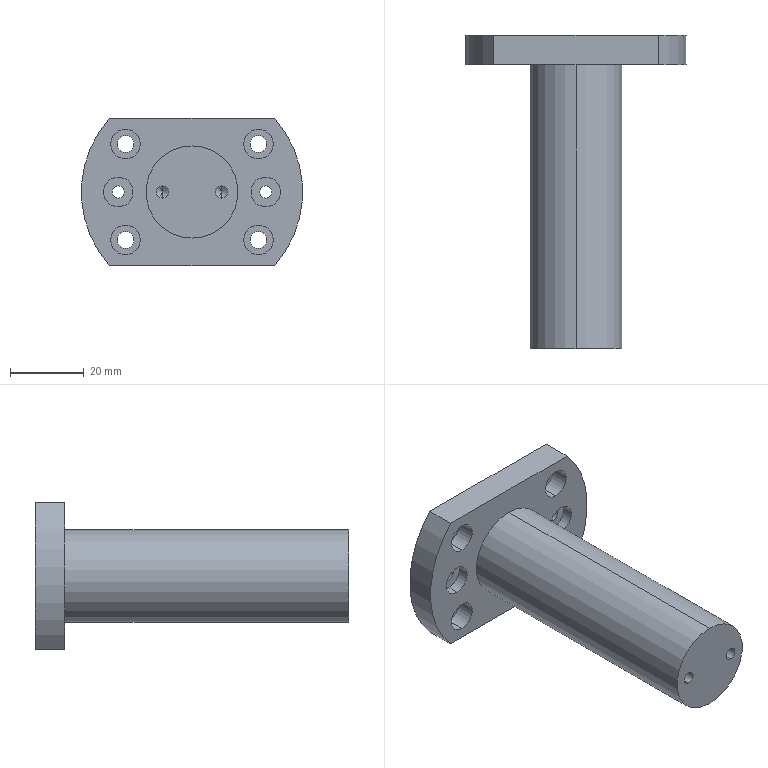Part | SolidWorks | features 3DProfileFeature 4, HoleWzd 4, ICE 1, Revolution 1 | 1 solid | 47 faces | box 60 x 85 x 40 mm | volume 53675 mm3 | cylinder 32 | plane 11 | cone 4 | commonest cylinder face diameters 8 x12 3.3 x8 4.5 x8 25 x2 60 x2
STEP:
#1=CARTESIAN_POINT('',(-18.,82.,17.));
#2=VERTEX_POINT('',#1);
#3=CARTESIAN_POINT('',(-18.,82.,9.));
#4=VERTEX_POINT('',#3);
#5=CARTESIAN_POINT('',(-18.,82.,13.));
#6=DIRECTION('',(0.,-1.,0.));
#7=DIRECTION('',(0.,0.,-1.));
#8=AXIS2_PLACEMENT_3D('',#5,#6,#7);
#9=CIRCLE('',#8,4.);
#10=EDGE_CURVE('',#2,#4,#9,.T.);
#11=ORIENTED_EDGE('',*,*,#10,.F.);
#12=CARTESIAN_POINT('',(-18.,77.,17.));
#13=VERTEX_POINT('',#12);
#14=CARTESIAN_POINT('',(-18.,77.,17.));
#15=DIRECTION('',(0.,-1.,0.));
#16=VECTOR('',#15,1000.);
#17=LINE('',#14,#16);
#18=EDGE_CURVE('',#2,#13,#17,.T.);
#19=ORIENTED_EDGE('',*,*,#18,.T.);
#20=CARTESIAN_POINT('',(-18.,77.,9.));
#21=VERTEX_POINT('',#20);
#22=CARTESIAN_POINT('',(-18.,77.,13.));
#23=DIRECTION('',(0.,-1.,0.));
#24=DIRECTION('',(0.,0.,-1.));
#25=AXIS2_PLACEMENT_3D('',#22,#23,#24);
#26=CIRCLE('',#25,4.);
#27=EDGE_CURVE('',#13,#21,#26,.T.);
#28=ORIENTED_EDGE('',*,*,#27,.T.);
#29=CARTESIAN_POINT('',(-18.,77.,9.));
#30=DIRECTION('',(0.,-1.,0.));
#31=VECTOR('',#30,1000.);
#32=LINE('',#29,#31);
#33=EDGE_CURVE('',#4,#21,#32,.T.);
#34=ORIENTED_EDGE('',*,*,#33,.F.);
#35=EDGE_LOOP('',(#11,#19,#28,#34));
#36=FACE_OUTER_BOUND('',#35,.T.);
#37=CARTESIAN_POINT('',(-18.,77.,13.));
#38=DIRECTION('',(0.,-1.,0.));
#39=DIRECTION('',(0.,0.,-1.));
#40=AXIS2_PLACEMENT_3D('',#37,#38,#39);
#41=CYLINDRICAL_SURFACE('',#40,4.);
#42=ADVANCED_FACE('',(#36),#41,.F.);
#43=CARTESIAN_POINT('',(-18.,85.,15.25));
#44=VERTEX_POINT('',#43);
#45=CARTESIAN_POINT('',(-18.,85.,10.75));
#46=VERTEX_POINT('',#45);
#47=CARTESIAN_POINT('',(-18.,85.,13.));
#48=DIRECTION('',(0.,-1.,0.));
#49=DIRECTION('',(0.,0.,-1.));
#50=AXIS2_PLACEMENT_3D('',#47,#48,#49);
#51=CIRCLE('',#50,2.25);
#52=EDGE_CURVE('',#44,#46,#51,.T.);
#53=ORIENTED_EDGE('',*,*,#52,.F.);
#54=CARTESIAN_POINT('',(-18.,82.,15.25));
#55=VERTEX_POINT('',#54);
#56=CARTESIAN_POINT('',(-18.,77.,15.25));
#57=DIRECTION('',(0.,-1.,0.));
#58=VECTOR('',#57,1000.);
#59=LINE('',#56,#58);
#60=EDGE_CURVE('',#44,#55,#59,.T.);
#61=ORIENTED_EDGE('',*,*,#60,.T.);
#62=CARTESIAN_POINT('',(-18.,82.,10.75));
#63=VERTEX_POINT('',#62);
#64=CARTESIAN_POINT('',(-18.,82.,13.));
#65=DIRECTION('',(0.,-1.,0.));
#66=DIRECTION('',(0.,0.,-1.));
#67=AXIS2_PLACEMENT_3D('',#64,#65,#66);
#68=CIRCLE('',#67,2.25);
#69=EDGE_CURVE('',#55,#63,#68,.T.);
#70=ORIENTED_EDGE('',*,*,#69,.T.);
#71=CARTESIAN_POINT('',(-18.,77.,10.75));
#72=DIRECTION('',(0.,-1.,0.));
#73=VECTOR('',#72,1000.);
#74=LINE('',#71,#73);
#75=EDGE_CURVE('',#46,#63,#74,.T.);
#76=ORIENTED_EDGE('',*,*,#75,.F.);
#77=EDGE_LOOP('',(#53,#61,#70,#76));
#78=FACE_OUTER_BOUND('',#77,.T.);
#79=CARTESIAN_POINT('',(-18.,77.,13.));
#80=DIRECTION('',(0.,-1.,0.));
#81=DIRECTION('',(0.,0.,-1.));
#82=AXIS2_PLACEMENT_3D('',#79,#80,#81);
#83=CYLINDRICAL_SURFACE('',#82,2.25);
#84=ADVANCED_FACE('',(#78),#83,.F.);
#85=CARTESIAN_POINT('',(18.,82.,17.));
#86=VERTEX_POINT('',#85);
#87=CARTESIAN_POINT('',(18.,82.,9.));
#88=VERTEX_POINT('',#87);
#89=CARTESIAN_POINT('',(18.,82.,13.));
#90=DIRECTION('',(0.,-1.,0.));
#91=DIRECTION('',(0.,0.,-1.));
#92=AXIS2_PLACEMENT_3D('',#89,#90,#91);
#93=CIRCLE('',#92,4.);
#94=EDGE_CURVE('',#86,#88,#93,.T.);
#95=ORIENTED_EDGE('',*,*,#94,.F.);
#96=CARTESIAN_POINT('',(18.,77.,17.));
#97=VERTEX_POINT('',#96);
#98=CARTESIAN_POINT('',(18.,77.,17.));
#99=DIRECTION('',(0.,-1.,0.));
#100=VECTOR('',#99,1000.);
#101=LINE('',#98,#100);
#102=EDGE_CURVE('',#86,#97,#101,.T.);
#103=ORIENTED_EDGE('',*,*,#102,.T.);
#104=CARTESIAN_POINT('',(18.,77.,9.));
#105=VERTEX_POINT('',#104);
#106=CARTESIAN_POINT('',(18.,77.,13.));
#107=DIRECTION('',(0.,-1.,0.));
#108=DIRECTION('',(0.,0.,-1.));
#109=AXIS2_PLACEMENT_3D('',#106,#107,#108);
#110=CIRCLE('',#109,4.);
#111=EDGE_CURVE('',#97,#105,#110,.T.);
#112=ORIENTED_EDGE('',*,*,#111,.T.);
#113=CARTESIAN_POINT('',(18.,77.,9.));
#114=DIRECTION('',(0.,-1.,0.));
#115=VECTOR('',#114,1000.);
#116=LINE('',#113,#115);
#117=EDGE_CURVE('',#88,#105,#116,.T.);
#118=ORIENTED_EDGE('',*,*,#117,.F.);
#119=EDGE_LOOP('',(#95,#103,#112,#118));
#120=FACE_OUTER_BOUND('',#119,.T.);
#121=CARTESIAN_POINT('',(18.,77.,13.));
#122=DIRECTION('',(0.,-1.,0.));
#123=DIRECTION('',(0.,0.,-1.));
#124=AXIS2_PLACEMENT_3D('',#121,#122,#123);
#125=CYLINDRICAL_SURFACE('',#124,4.);
#126=ADVANCED_FACE('',(#120),#125,.F.);
#127=CARTESIAN_POINT('',(18.,85.,15.25));
#128=VERTEX_POINT('',#127);
#129=CARTESIAN_POINT('',(18.,85.,10.75));
#130=VERTEX_POINT('',#129);
#131=CARTESIAN_POINT('',(18.,85.,13.));
#132=DIRECTION('',(0.,-1.,0.));
#133=DIRECTION('',(0.,0.,-1.));
#134=AXIS2_PLACEMENT_3D('',#131,#132,#133);
#135=CIRCLE('',#134,2.25);
#136=EDGE_CURVE('',#128,#130,#135,.T.);
#137=ORIENTED_EDGE('',*,*,#136,.F.);
#138=CARTESIAN_POINT('',(18.,82.,15.25));
#139=VERTEX_POINT('',#138);
#140=CARTESIAN_POINT('',(18.,77.,15.25));
#141=DIRECTION('',(0.,-1.,0.));
#142=VECTOR('',#141,1000.);
#143=LINE('',#140,#142);
#144=EDGE_CURVE('',#128,#139,#143,.T.);
#145=ORIENTED_EDGE('',*,*,#144,.T.);
#146=CARTESIAN_POINT('',(18.,82.,10.75));
#147=VERTEX_POINT('',#146);
#148=CARTESIAN_POINT('',(18.,82.,13.));
#149=DIRECTION('',(0.,-1.,0.));
#150=DIRECTION('',(0.,0.,-1.));
#151=AXIS2_PLACEMENT_3D('',#148,#149,#150);
#152=CIRCLE('',#151,2.25);
#153=EDGE_CURVE('',#139,#147,#152,.T.);
#154=ORIENTED_EDGE('',*,*,#153,.T.);
#155=CARTESIAN_POINT('',(18.,77.,10.75));
#156=DIRECTION('',(0.,-1.,0.));
#157=VECTOR('',#156,1000.);
#158=LINE('',#155,#157);
#159=EDGE_CURVE('',#130,#147,#158,.T.);
#160=ORIENTED_EDGE('',*,*,#159,.F.);
#161=EDGE_LOOP('',(#137,#145,#154,#160));
#162=FACE_OUTER_BOUND('',#161,.T.);
#163=CARTESIAN_POINT('',(18.,77.,13.));
#164=DIRECTION('',(0.,-1.,0.));
#165=DIRECTION('',(0.,0.,-1.));
#166=AXIS2_PLACEMENT_3D('',#163,#164,#165);
#167=CYLINDRICAL_SURFACE('',#166,2.25);
#168=ADVANCED_FACE('',(#162),#167,.F.);
#169=CARTESIAN_POINT('',(18.,82.,-9.));
#170=VERTEX_POINT('',#169);
#171=CARTESIAN_POINT('',(18.,82.,-17.));
#172=VERTEX_POINT('',#171);
#173=CARTESIAN_POINT('',(18.,82.,-13.));
#174=DIRECTION('',(0.,-1.,0.));
#175=DIRECTION('',(0.,0.,-1.));
#176=AXIS2_PLACEMENT_3D('',#173,#174,#175);
#177=CIRCLE('',#176,4.);
#178=EDGE_CURVE('',#170,#172,#177,.T.);
#179=ORIENTED_EDGE('',*,*,#178,.F.);
#180=CARTESIAN_POINT('',(18.,77.,-9.));
#181=VERTEX_POINT('',#180);
#182=CARTESIAN_POINT('',(18.,77.,-9.));
#183=DIRECTION('',(0.,-1.,0.));
#184=VECTOR('',#183,1000.);
#185=LINE('',#182,#184);
#186=EDGE_CURVE('',#170,#181,#185,.T.);
#187=ORIENTED_EDGE('',*,*,#186,.T.);
#188=CARTESIAN_POINT('',(18.,77.,-17.));
#189=VERTEX_POINT('',#188);
#190=CARTESIAN_POINT('',(18.,77.,-13.));
#191=DIRECTION('',(0.,-1.,0.));
#192=DIRECTION('',(0.,0.,-1.));
#193=AXIS2_PLACEMENT_3D('',#190,#191,#192);
#194=CIRCLE('',#193,4.);
#195=EDGE_CURVE('',#181,#189,#194,.T.);
#196=ORIENTED_EDGE('',*,*,#195,.T.);
#197=CARTESIAN_POINT('',(18.,77.,-17.));
#198=DIRECTION('',(0.,-1.,0.));
#199=VECTOR('',#198,1000.);
#200=LINE('',#197,#199);
#201=EDGE_CURVE('',#172,#189,#200,.T.);
#202=ORIENTED_EDGE('',*,*,#201,.F.);
#203=EDGE_LOOP('',(#179,#187,#196,#202));
#204=FACE_OUTER_BOUND('',#203,.T.);
#205=CARTESIAN_POINT('',(18.,77.,-13.));
#206=DIRECTION('',(0.,-1.,0.));
#207=DIRECTION('',(0.,0.,-1.));
#208=AXIS2_PLACEMENT_3D('',#205,#206,#207);
#209=CYLINDRICAL_SURFACE('',#208,4.);
#210=ADVANCED_FACE('',(#204),#209,.F.);
#211=CARTESIAN_POINT('',(18.,85.,-10.75));
#212=VERTEX_POINT('',#211);
#213=CARTESIAN_POINT('',(18.,85.,-15.25));
#214=VERTEX_POINT('',#213);
#215=CARTESIAN_POINT('',(18.,85.,-13.));
#216=DIRECTION('',(0.,-1.,0.));
#217=DIRECTION('',(0.,0.,-1.));
#218=AXIS2_PLACEMENT_3D('',#215,#216,#217);
#219=CIRCLE('',#218,2.25);
#220=EDGE_CURVE('',#212,#214,#219,.T.);
#221=ORIENTED_EDGE('',*,*,#220,.F.);
#222=CARTESIAN_POINT('',(18.,82.,-10.75));
#223=VERTEX_POINT('',#222);
#224=CARTESIAN_POINT('',(18.,77.,-10.75));
#225=DIRECTION('',(0.,-1.,0.));
#226=VECTOR('',#225,1000.);
#227=LINE('',#224,#226);
#228=EDGE_CURVE('',#212,#223,#227,.T.);
#229=ORIENTED_EDGE('',*,*,#228,.T.);
#230=CARTESIAN_POINT('',(18.,82.,-15.25));
#231=VERTEX_POINT('',#230);
#232=CARTESIAN_POINT('',(18.,82.,-13.));
#233=DIRECTION('',(0.,-1.,0.));
#234=DIRECTION('',(0.,0.,-1.));
#235=AXIS2_PLACEMENT_3D('',#232,#233,#234);
#236=CIRCLE('',#235,2.25);
#237=EDGE_CURVE('',#223,#231,#236,.T.);
#238=ORIENTED_EDGE('',*,*,#237,.T.);
#239=CARTESIAN_POINT('',(18.,77.,-15.25));
#240=DIRECTION('',(0.,-1.,0.));
#241=VECTOR('',#240,1000.);
#242=LINE('',#239,#241);
#243=EDGE_CURVE('',#214,#231,#242,.T.);
#244=ORIENTED_EDGE('',*,*,#243,.F.);
#245=EDGE_LOOP('',(#221,#229,#238,#244));
#246=FACE_OUTER_BOUND('',#245,.T.);
#247=CARTESIAN_POINT('',(18.,77.,-13.));
#248=DIRECTION('',(0.,-1.,0.));
#249=DIRECTION('',(0.,0.,-1.));
#250=AXIS2_PLACEMENT_3D('',#247,#248,#249);
#251=CYLINDRICAL_SURFACE('',#250,2.25);
#252=ADVANCED_FACE('',(#246),#251,.F.);
#253=CARTESIAN_POINT('',(-18.,82.,-9.));
#254=VERTEX_POINT('',#253);
#255=CARTESIAN_POINT('',(-18.,82.,-17.));
#256=VERTEX_POINT('',#255);
#257=CARTESIAN_POINT('',(-18.,82.,-13.));
#258=DIRECTION('',(0.,-1.,0.));
#259=DIRECTION('',(0.,0.,-1.));
#260=AXIS2_PLACEMENT_3D('',#257,#258,#259);
#261=CIRCLE('',#260,4.);
#262=EDGE_CURVE('',#254,#256,#261,.T.);
#263=ORIENTED_EDGE('',*,*,#262,.F.);
#264=CARTESIAN_POINT('',(-18.,77.,-9.));
#265=VERTEX_POINT('',#264);
#266=CARTESIAN_POINT('',(-18.,77.,-9.));
#267=DIRECTION('',(0.,-1.,0.));
#268=VECTOR('',#267,1000.);
#269=LINE('',#266,#268);
#270=EDGE_CURVE('',#254,#265,#269,.T.);
#271=ORIENTED_EDGE('',*,*,#270,.T.);
#272=CARTESIAN_POINT('',(-18.,77.,-17.));
#273=VERTEX_POINT('',#272);
#274=CARTESIAN_POINT('',(-18.,77.,-13.));
#275=DIRECTION('',(0.,-1.,0.));
#276=DIRECTION('',(0.,0.,-1.));
#277=AXIS2_PLACEMENT_3D('',#274,#275,#276);
#278=CIRCLE('',#277,4.);
#279=EDGE_CURVE('',#265,#273,#278,.T.);
#280=ORIENTED_EDGE('',*,*,#279,.T.);
#281=CARTESIAN_POINT('',(-18.,77.,-17.));
#282=DIRECTION('',(0.,-1.,0.));
#283=VECTOR('',#282,1000.);
#284=LINE('',#281,#283);
#285=EDGE_CURVE('',#256,#273,#284,.T.);
#286=ORIENTED_EDGE('',*,*,#285,.F.);
#287=EDGE_LOOP('',(#263,#271,#280,#286));
#288=FACE_OUTER_BOUND('',#287,.T.);
#289=CARTESIAN_POINT('',(-18.,77.,-13.));
#290=DIRECTION('',(0.,-1.,0.));
#291=DIRECTION('',(0.,0.,-1.));
#292=AXIS2_PLACEMENT_3D('',#289,#290,#291);
#293=CYLINDRICAL_SURFACE('',#292,4.);
#294=ADVANCED_FACE('',(#288),#293,.F.);
#295=CARTESIAN_POINT('',(-18.,85.,-10.75));
#296=VERTEX_POINT('',#295);
#297=CARTESIAN_POINT('',(-18.,85.,-15.25));
#298=VERTEX_POINT('',#297);
#299=CARTESIAN_POINT('',(-18.,85.,-13.));
#300=DIRECTION('',(0.,-1.,0.));
#301=DIRECTION('',(0.,0.,-1.));
#302=AXIS2_PLACEMENT_3D('',#299,#300,#301);
#303=CIRCLE('',#302,2.25);
#304=EDGE_CURVE('',#296,#298,#303,.T.);
#305=ORIENTED_EDGE('',*,*,#304,.F.);
#306=CARTESIAN_POINT('',(-18.,82.,-10.75));
#307=VERTEX_POINT('',#306);
#308=CARTESIAN_POINT('',(-18.,77.,-10.75));
#309=DIRECTION('',(0.,-1.,0.));
#310=VECTOR('',#309,1000.);
#311=LINE('',#308,#310);
#312=EDGE_CURVE('',#296,#307,#311,.T.);
#313=ORIENTED_EDGE('',*,*,#312,.T.);
#314=CARTESIAN_POINT('',(-18.,82.,-15.25));
#315=VERTEX_POINT('',#314);
#316=CARTESIAN_POINT('',(-18.,82.,-13.));
#317=DIRECTION('',(0.,-1.,0.));
#318=DIRECTION('',(0.,0.,-1.));
#319=AXIS2_PLACEMENT_3D('',#316,#317,#318);
#320=CIRCLE('',#319,2.25);
#321=EDGE_CURVE('',#307,#315,#320,.T.);
#322=ORIENTED_EDGE('',*,*,#321,.T.);
#323=CARTESIAN_POINT('',(-18.,77.,-15.25));
#324=DIRECTION('',(0.,-1.,0.));
#325=VECTOR('',#324,1000.);
#326=LINE('',#323,#325);
#327=EDGE_CURVE('',#298,#315,#326,.T.);
#328=ORIENTED_EDGE('',*,*,#327,.F.);
#329=EDGE_LOOP('',(#305,#313,#322,#328));
#330=FACE_OUTER_BOUND('',#329,.T.);
#331=CARTESIAN_POINT('',(-18.,77.,-13.));
#332=DIRECTION('',(0.,-1.,0.));
#333=DIRECTION('',(0.,0.,-1.));
#334=AXIS2_PLACEMENT_3D('',#331,#332,#333);
#335=CYLINDRICAL_SURFACE('',#334,2.25);
#336=ADVANCED_FACE('',(#330),#335,.F.);
#337=CARTESIAN_POINT('',(-20.,85.,1.65));
#338=VERTEX_POINT('',#337);
#339=CARTESIAN_POINT('',(-20.,85.,-1.65));
#340=VERTEX_POINT('',#339);
#341=CARTESIAN_POINT('',(-20.,85.,0.));
#342=DIRECTION('',(0.,-1.,0.));
#343=DIRECTION('',(0.,0.,-1.));
#344=AXIS2_PLACEMENT_3D('',#341,#342,#343);
#345=CIRCLE('',#344,1.65);
#346=EDGE_CURVE('',#338,#340,#345,.T.);
#347=ORIENTED_EDGE('',*,*,#346,.F.);
#348=CARTESIAN_POINT('',(-20.,80.,1.65));
#349=VERTEX_POINT('',#348);
#350=CARTESIAN_POINT('',(-20.,80.,1.65));
#351=DIRECTION('',(0.,-1.,0.));
#352=VECTOR('',#351,1000.);
#353=LINE('',#350,#352);
#354=EDGE_CURVE('',#338,#349,#353,.T.);
#355=ORIENTED_EDGE('',*,*,#354,.T.);
#356=CARTESIAN_POINT('',(-20.,80.,-1.65));
#357=VERTEX_POINT('',#356);
#358=CARTESIAN_POINT('',(-20.,80.,0.));
#359=DIRECTION('',(0.,-1.,0.));
#360=DIRECTION('',(0.,0.,-1.));
#361=AXIS2_PLACEMENT_3D('',#358,#359,#360);
#362=CIRCLE('',#361,1.65);
#363=EDGE_CURVE('',#349,#357,#362,.T.);
#364=ORIENTED_EDGE('',*,*,#363,.T.);
#365=CARTESIAN_POINT('',(-20.,80.,-1.65));
#366=DIRECTION('',(0.,-1.,0.));
#367=VECTOR('',#366,1000.);
#368=LINE('',#365,#367);
#369=EDGE_CURVE('',#340,#357,#368,.T.);
#370=ORIENTED_EDGE('',*,*,#369,.F.);
#371=EDGE_LOOP('',(#347,#355,#364,#370));
#372=FACE_OUTER_BOUND('',#371,.T.);
#373=CARTESIAN_POINT('',(-20.,80.,0.));
#374=DIRECTION('',(0.,-1.,0.));
#375=DIRECTION('',(0.,0.,-1.));
#376=AXIS2_PLACEMENT_3D('',#373,#374,#375);
#377=CYLINDRICAL_SURFACE('',#376,1.65);
#378=ADVANCED_FACE('',(#372),#377,.F.);
#379=CARTESIAN_POINT('',(20.,85.,1.65));
#380=VERTEX_POINT('',#379);
#381=CARTESIAN_POINT('',(20.,85.,-1.65));
#382=VERTEX_POINT('',#381);
#383=CARTESIAN_POINT('',(20.,85.,0.));
#384=DIRECTION('',(0.,-1.,0.));
#385=DIRECTION('',(0.,0.,-1.));
#386=AXIS2_PLACEMENT_3D('',#383,#384,#385);
#387=CIRCLE('',#386,1.65);
#388=EDGE_CURVE('',#380,#382,#387,.T.);
#389=ORIENTED_EDGE('',*,*,#388,.F.);
#390=CARTESIAN_POINT('',(20.,80.,1.65));
#391=VERTEX_POINT('',#390);
#392=CARTESIAN_POINT('',(20.,80.,1.65));
#393=DIRECTION('',(0.,-1.,0.));
#394=VECTOR('',#393,1000.);
#395=LINE('',#392,#394);
#396=EDGE_CURVE('',#380,#391,#395,.T.);
#397=ORIENTED_EDGE('',*,*,#396,.T.);
#398=CARTESIAN_POINT('',(20.,80.,-1.65));
#399=VERTEX_POINT('',#398);
#400=CARTESIAN_POINT('',(20.,80.,0.));
#401=DIRECTION('',(0.,-1.,0.));
#402=DIRECTION('',(0.,0.,-1.));
#403=AXIS2_PLACEMENT_3D('',#400,#401,#402);
#404=CIRCLE('',#403,1.65);
#405=EDGE_CURVE('',#391,#399,#404,.T.);
#406=ORIENTED_EDGE('',*,*,#405,.T.);
#407=CARTESIAN_POINT('',(20.,80.,-1.65));
#408=DIRECTION('',(0.,-1.,0.));
#409=VECTOR('',#408,1000.);
#410=LINE('',#407,#409);
#411=EDGE_CURVE('',#382,#399,#410,.T.);
#412=ORIENTED_EDGE('',*,*,#411,.F.);
#413=EDGE_LOOP('',(#389,#397,#406,#412));
#414=FACE_OUTER_BOUND('',#413,.T.);
#415=CARTESIAN_POINT('',(20.,80.,0.));
#416=DIRECTION('',(0.,-1.,0.));
#417=DIRECTION('',(0.,0.,-1.));
#418=AXIS2_PLACEMENT_3D('',#415,#416,#417);
#419=CYLINDRICAL_SURFACE('',#418,1.65);
#420=ADVANCED_FACE('',(#414),#419,.F.);
#421=CARTESIAN_POINT('',(-20.,80.,4.));
#422=VERTEX_POINT('',#421);
#423=CARTESIAN_POINT('',(-20.,80.,-4.));
#424=VERTEX_POINT('',#423);
#425=CARTESIAN_POINT('',(-20.,80.,0.));
#426=DIRECTION('',(0.,-1.,0.));
#427=DIRECTION('',(0.,0.,-1.));
#428=AXIS2_PLACEMENT_3D('',#425,#426,#427);
#429=CIRCLE('',#428,4.);
#430=EDGE_CURVE('',#422,#424,#429,.T.);
#431=ORIENTED_EDGE('',*,*,#430,.F.);
#432=CARTESIAN_POINT('',(-20.,77.,4.));
#433=VERTEX_POINT('',#432);
#434=CARTESIAN_POINT('',(-20.,77.,4.));
#435=DIRECTION('',(0.,-1.,0.));
#436=VECTOR('',#435,1000.);
#437=LINE('',#434,#436);
#438=EDGE_CURVE('',#422,#433,#437,.T.);
#439=ORIENTED_EDGE('',*,*,#438,.T.);
#440=CARTESIAN_POINT('',(-20.,77.,-4.));
#441=VERTEX_POINT('',#440);
#442=CARTESIAN_POINT('',(-20.,77.,0.));
#443=DIRECTION('',(0.,-1.,0.));
#444=DIRECTION('',(0.,0.,-1.));
#445=AXIS2_PLACEMENT_3D('',#442,#443,#444);
#446=CIRCLE('',#445,4.);
#447=EDGE_CURVE('',#433,#441,#446,.T.);
#448=ORIENTED_EDGE('',*,*,#447,.T.);
#449=CARTESIAN_POINT('',(-20.,77.,-4.));
#450=DIRECTION('',(0.,-1.,0.));
#451=VECTOR('',#450,1000.);
#452=LINE('',#449,#451);
#453=EDGE_CURVE('',#424,#441,#452,.T.);
#454=ORIENTED_EDGE('',*,*,#453,.F.);
#455=EDGE_LOOP('',(#431,#439,#448,#454));
#456=FACE_OUTER_BOUND('',#455,.T.);
#457=CARTESIAN_POINT('',(-20.,77.,0.));
#458=DIRECTION('',(0.,-1.,0.));
#459=DIRECTION('',(0.,0.,-1.));
#460=AXIS2_PLACEMENT_3D('',#457,#458,#459);
#461=CYLINDRICAL_SURFACE('',#460,4.);
#462=ADVANCED_FACE('',(#456),#461,.F.);
#463=CARTESIAN_POINT('',(20.,80.,4.));
#464=VERTEX_POINT('',#463);
#465=CARTESIAN_POINT('',(20.,80.,-4.));
#466=VERTEX_POINT('',#465);
#467=CARTESIAN_POINT('',(20.,80.,0.));
#468=DIRECTION('',(0.,-1.,0.));
#469=DIRECTION('',(0.,0.,-1.));
#470=AXIS2_PLACEMENT_3D('',#467,#468,#469);
#471=CIRCLE('',#470,4.);
#472=EDGE_CURVE('',#464,#466,#471,.T.);
#473=ORIENTED_EDGE('',*,*,#472,.F.);
#474=CARTESIAN_POINT('',(20.,77.,4.));
#475=VERTEX_POINT('',#474);
#476=CARTESIAN_POINT('',(20.,77.,4.));
#477=DIRECTION('',(0.,-1.,0.));
#478=VECTOR('',#477,1000.);
#479=LINE('',#476,#478);
#480=EDGE_CURVE('',#464,#475,#479,.T.);
#481=ORIENTED_EDGE('',*,*,#480,.T.);
#482=CARTESIAN_POINT('',(20.,77.,-4.));
#483=VERTEX_POINT('',#482);
#484=CARTESIAN_POINT('',(20.,77.,0.));
#485=DIRECTION('',(0.,-1.,0.));
#486=DIRECTION('',(0.,0.,-1.));
#487=AXIS2_PLACEMENT_3D('',#484,#485,#486);
#488=CIRCLE('',#487,4.);
#489=EDGE_CURVE('',#475,#483,#488,.T.);
#490=ORIENTED_EDGE('',*,*,#489,.T.);
#491=CARTESIAN_POINT('',(20.,77.,-4.));
#492=DIRECTION('',(0.,-1.,0.));
#493=VECTOR('',#492,1000.);
#494=LINE('',#491,#493);
#495=EDGE_CURVE('',#466,#483,#494,.T.);
#496=ORIENTED_EDGE('',*,*,#495,.F.);
#497=EDGE_LOOP('',(#473,#481,#490,#496));
#498=FACE_OUTER_BOUND('',#497,.T.);
#499=CARTESIAN_POINT('',(20.,77.,0.));
#500=DIRECTION('',(0.,-1.,0.));
#501=DIRECTION('',(0.,0.,-1.));
#502=AXIS2_PLACEMENT_3D('',#499,#500,#501);
#503=CYLINDRICAL_SURFACE('',#502,4.);
#504=ADVANCED_FACE('',(#498),#503,.F.);
#505=CARTESIAN_POINT('',(-8.,11.5,1.65));
#506=VERTEX_POINT('',#505);
#507=CARTESIAN_POINT('',(-8.,11.5,-1.65));
#508=VERTEX_POINT('',#507);
#509=CARTESIAN_POINT('',(-8.,11.5,0.));
#510=DIRECTION('',(0.,-1.,0.));
#511=DIRECTION('',(0.,0.,-1.));
#512=AXIS2_PLACEMENT_3D('',#509,#510,#511);
#513=CIRCLE('',#512,1.65);
#514=EDGE_CURVE('',#506,#508,#513,.T.);
#515=ORIENTED_EDGE('',*,*,#514,.F.);
#516=CARTESIAN_POINT('',(-8.,0.,1.65));
#517=VERTEX_POINT('',#516);
#518=CARTESIAN_POINT('',(-8.,0.,1.65));
#519=DIRECTION('',(0.,-1.,0.));
#520=VECTOR('',#519,1000.);
#521=LINE('',#518,#520);
#522=EDGE_CURVE('',#506,#517,#521,.T.);
#523=ORIENTED_EDGE('',*,*,#522,.T.);
#524=CARTESIAN_POINT('',(-8.,0.,-1.65));
#525=VERTEX_POINT('',#524);
#526=CARTESIAN_POINT('',(-8.,0.,0.));
#527=DIRECTION('',(0.,-1.,0.));
#528=DIRECTION('',(0.,0.,-1.));
#529=AXIS2_PLACEMENT_3D('',#526,#527,#528);
#530=CIRCLE('',#529,1.65);
#531=EDGE_CURVE('',#517,#525,#530,.T.);
#532=ORIENTED_EDGE('',*,*,#531,.T.);
#533=CARTESIAN_POINT('',(-8.,0.,-1.65));
#534=DIRECTION('',(0.,-1.,0.));
#535=VECTOR('',#534,1000.);
#536=LINE('',#533,#535);
#537=EDGE_CURVE('',#508,#525,#536,.T.);
#538=ORIENTED_EDGE('',*,*,#537,.F.);
#539=EDGE_LOOP('',(#515,#523,#532,#538));
#540=FACE_OUTER_BOUND('',#539,.T.);
#541=CARTESIAN_POINT('',(-8.,0.,0.));
#542=DIRECTION('',(0.,-1.,0.));
#543=DIRECTION('',(0.,0.,-1.));
#544=AXIS2_PLACEMENT_3D('',#541,#542,#543);
#545=CYLINDRICAL_SURFACE('',#544,1.65);
#546=ADVANCED_FACE('',(#540),#545,.F.);
#547=CARTESIAN_POINT('',(-8.,12.491,0.));
#548=VERTEX_POINT('',#547);
#549=CARTESIAN_POINT('',(-8.,11.5,-1.65));
#550=DIRECTION('',(0.,-0.515,-0.8572));
#551=VECTOR('',#550,1000.);
#552=LINE('',#549,#551);
#553=EDGE_CURVE('',#548,#508,#552,.T.);
#554=ORIENTED_EDGE('',*,*,#553,.F.);
#555=CARTESIAN_POINT('',(-8.,11.5,1.65));
#556=DIRECTION('',(0.,-0.515,0.8572));
#557=VECTOR('',#556,1000.);
#558=LINE('',#555,#557);
#559=EDGE_CURVE('',#548,#506,#558,.T.);
#560=ORIENTED_EDGE('',*,*,#559,.T.);
#561=ORIENTED_EDGE('',*,*,#514,.T.);
#562=EDGE_LOOP('',(#554,#560,#561));
#563=FACE_OUTER_BOUND('',#562,.T.);
#564=CARTESIAN_POINT('',(-8.,11.5,0.));
#565=DIRECTION('',(0.,-1.,0.));
#566=DIRECTION('',(0.,0.,-1.));
#567=AXIS2_PLACEMENT_3D('',#564,#565,#566);
#568=CONICAL_SURFACE('',#567,1.65,1.03);
#569=ADVANCED_FACE('',(#563),#568,.F.);
#570=CARTESIAN_POINT('',(8.,11.5,1.65));
#571=VERTEX_POINT('',#570);
#572=CARTESIAN_POINT('',(8.,11.5,-1.65));
#573=VERTEX_POINT('',#572);
#574=CARTESIAN_POINT('',(8.,11.5,0.));
#575=DIRECTION('',(0.,-1.,0.));
#576=DIRECTION('',(0.,0.,-1.));
#577=AXIS2_PLACEMENT_3D('',#574,#575,#576);
#578=CIRCLE('',#577,1.65);
#579=EDGE_CURVE('',#571,#573,#578,.T.);
#580=ORIENTED_EDGE('',*,*,#579,.F.);
#581=CARTESIAN_POINT('',(8.,0.,1.65));
#582=VERTEX_POINT('',#581);
#583=CARTESIAN_POINT('',(8.,0.,1.65));
#584=DIRECTION('',(0.,-1.,0.));
#585=VECTOR('',#584,1000.);
#586=LINE('',#583,#585);
#587=EDGE_CURVE('',#571,#582,#586,.T.);
#588=ORIENTED_EDGE('',*,*,#587,.T.);
#589=CARTESIAN_POINT('',(8.,0.,-1.65));
#590=VERTEX_POINT('',#589);
#591=CARTESIAN_POINT('',(8.,0.,0.));
#592=DIRECTION('',(0.,-1.,0.));
#593=DIRECTION('',(0.,0.,-1.));
#594=AXIS2_PLACEMENT_3D('',#591,#592,#593);
#595=CIRCLE('',#594,1.65);
#596=EDGE_CURVE('',#582,#590,#595,.T.);
#597=ORIENTED_EDGE('',*,*,#596,.T.);
#598=CARTESIAN_POINT('',(8.,0.,-1.65));
#599=DIRECTION('',(0.,-1.,0.));
#600=VECTOR('',#599,1000.);
#601=LINE('',#598,#600);
#602=EDGE_CURVE('',#573,#590,#601,.T.);
#603=ORIENTED_EDGE('',*,*,#602,.F.);
#604=EDGE_LOOP('',(#580,#588,#597,#603));
#605=FACE_OUTER_BOUND('',#604,.T.);
#606=CARTESIAN_POINT('',(8.,0.,0.));
#607=DIRECTION('',(0.,-1.,0.));
#608=DIRECTION('',(0.,0.,-1.));
#609=AXIS2_PLACEMENT_3D('',#606,#607,#608);
#610=CYLINDRICAL_SURFACE('',#609,1.65);
#611=ADVANCED_FACE('',(#605),#610,.F.);
#612=CARTESIAN_POINT('',(8.,12.491,0.));
#613=VERTEX_POINT('',#612);
#614=CARTESIAN_POINT('',(8.,11.5,-1.65));
#615=DIRECTION('',(0.,-0.515,-0.8572));
#616=VECTOR('',#615,1000.);
#617=LINE('',#614,#616);
#618=EDGE_CURVE('',#613,#573,#617,.T.);
#619=ORIENTED_EDGE('',*,*,#618,.F.);
#620=CARTESIAN_POINT('',(8.,11.5,1.65));
#621=DIRECTION('',(0.,-0.515,0.8572));
#622=VECTOR('',#621,1000.);
#623=LINE('',#620,#622);
#624=EDGE_CURVE('',#613,#571,#623,.T.);
#625=ORIENTED_EDGE('',*,*,#624,.T.);
#626=ORIENTED_EDGE('',*,*,#579,.T.);
#627=EDGE_LOOP('',(#619,#625,#626));
#628=FACE_OUTER_BOUND('',#627,.T.);
#629=CARTESIAN_POINT('',(8.,11.5,0.));
#630=DIRECTION('',(0.,-1.,0.));
#631=DIRECTION('',(0.,0.,-1.));
#632=AXIS2_PLACEMENT_3D('',#629,#630,#631);
#633=CONICAL_SURFACE('',#632,1.65,1.03);
#634=ADVANCED_FACE('',(#628),#633,.F.);
#635=CARTESIAN_POINT('',(0.,77.,-12.5));
#636=VERTEX_POINT('',#635);
#637=CARTESIAN_POINT('',(0.,77.,12.5));
#638=VERTEX_POINT('',#637);
#639=CARTESIAN_POINT('',(0.,77.,0.));
#640=DIRECTION('',(0.,-1.,0.));
#641=DIRECTION('',(0.,0.,-1.));
#642=AXIS2_PLACEMENT_3D('',#639,#640,#641);
#643=CIRCLE('',#642,12.5);
#644=EDGE_CURVE('',#636,#638,#643,.T.);
#645=ORIENTED_EDGE('',*,*,#644,.T.);
#646=CARTESIAN_POINT('',(0.,0.,12.5));
#647=VERTEX_POINT('',#646);
#648=CARTESIAN_POINT('',(0.,0.,12.5));
#649=DIRECTION('',(0.,-1.,0.));
#650=VECTOR('',#649,1000.);
#651=LINE('',#648,#650);
#652=EDGE_CURVE('',#638,#647,#651,.T.);
#653=ORIENTED_EDGE('',*,*,#652,.T.);
#654=CARTESIAN_POINT('',(0.,0.,-12.5));
#655=VERTEX_POINT('',#654);
#656=CARTESIAN_POINT('',(0.,0.,0.));
#657=DIRECTION('',(0.,-1.,0.));
#658=DIRECTION('',(0.,0.,-1.));
#659=AXIS2_PLACEMENT_3D('',#656,#657,#658);
#660=CIRCLE('',#659,12.5);
#661=EDGE_CURVE('',#655,#647,#660,.T.);
#662=ORIENTED_EDGE('',*,*,#661,.F.);
#663=CARTESIAN_POINT('',(0.,0.,-12.5));
#664=DIRECTION('',(0.,-1.,0.));
#665=VECTOR('',#664,1000.);
#666=LINE('',#663,#665);
#667=EDGE_CURVE('',#636,#655,#666,.T.);
#668=ORIENTED_EDGE('',*,*,#667,.F.);
#669=EDGE_LOOP('',(#645,#653,#662,#668));
#670=FACE_OUTER_BOUND('',#669,.T.);
#671=CARTESIAN_POINT('',(0.,0.,0.));
#672=DIRECTION('',(0.,-1.,0.));
#673=DIRECTION('',(0.,0.,-1.));
#674=AXIS2_PLACEMENT_3D('',#671,#672,#673);
#675=CYLINDRICAL_SURFACE('',#674,12.5);
#676=ADVANCED_FACE('',(#670),#675,.T.);
#677=CARTESIAN_POINT('',(-20.,80.,0.));
#678=DIRECTION('',(0.,-1.,0.));
#679=DIRECTION('',(0.,0.,-1.));
#680=AXIS2_PLACEMENT_3D('',#677,#678,#679);
#681=CIRCLE('',#680,4.);
#682=EDGE_CURVE('',#424,#422,#681,.T.);
#683=ORIENTED_EDGE('',*,*,#682,.T.);
#684=ORIENTED_EDGE('',*,*,#430,.T.);
#685=EDGE_LOOP('',(#683,#684));
#686=FACE_OUTER_BOUND('',#685,.T.);
#687=CARTESIAN_POINT('',(-20.,80.,0.));
#688=DIRECTION('',(0.,-1.,0.));
#689=DIRECTION('',(0.,0.,-1.));
#690=AXIS2_PLACEMENT_3D('',#687,#688,#689);
#691=CIRCLE('',#690,1.65);
#692=EDGE_CURVE('',#357,#349,#691,.T.);
#693=ORIENTED_EDGE('',*,*,#692,.F.);
#694=ORIENTED_EDGE('',*,*,#363,.F.);
#695=EDGE_LOOP('',(#693,#694));
#696=FACE_BOUND('',#695,.T.);
#697=CARTESIAN_POINT('',(-18.5,80.,0.));
#698=DIRECTION('',(0.,1.,0.));
#699=DIRECTION('',(0.,0.,1.));
#700=AXIS2_PLACEMENT_3D('',#697,#698,#699);
#701=PLANE('',#700);
#702=ADVANCED_FACE('',(#686,#696),#701,.F.);
#703=CARTESIAN_POINT('',(-18.,77.,13.));
#704=DIRECTION('',(0.,-1.,0.));
#705=DIRECTION('',(0.,0.,-1.));
#706=AXIS2_PLACEMENT_3D('',#703,#704,#705);
#707=CIRCLE('',#706,4.);
#708=EDGE_CURVE('',#21,#13,#707,.T.);
#709=ORIENTED_EDGE('',*,*,#708,.F.);
#710=ORIENTED_EDGE('',*,*,#27,.F.);
#711=EDGE_LOOP('',(#709,#710));
#712=FACE_BOUND('',#711,.T.);
#713=CARTESIAN_POINT('',(18.,77.,13.));
#714=DIRECTION('',(0.,-1.,0.));
#715=DIRECTION('',(0.,0.,-1.));
#716=AXIS2_PLACEMENT_3D('',#713,#714,#715);
#717=CIRCLE('',#716,4.);
#718=EDGE_CURVE('',#105,#97,#717,.T.);
#719=ORIENTED_EDGE('',*,*,#718,.F.);
#720=ORIENTED_EDGE('',*,*,#111,.F.);
#721=EDGE_LOOP('',(#719,#720));
#722=FACE_BOUND('',#721,.T.);
#723=CARTESIAN_POINT('',(18.,77.,-13.));
#724=DIRECTION('',(0.,-1.,0.));
#725=DIRECTION('',(0.,0.,-1.));
#726=AXIS2_PLACEMENT_3D('',#723,#724,#725);
#727=CIRCLE('',#726,4.);
#728=EDGE_CURVE('',#189,#181,#727,.T.);
#729=ORIENTED_EDGE('',*,*,#728,.F.);
#730=ORIENTED_EDGE('',*,*,#195,.F.);
#731=EDGE_LOOP('',(#729,#730));
#732=FACE_BOUND('',#731,.T.);
#733=CARTESIAN_POINT('',(-18.,77.,-13.));
#734=DIRECTION('',(0.,-1.,0.));
#735=DIRECTION('',(0.,0.,-1.));
#736=AXIS2_PLACEMENT_3D('',#733,#734,#735);
#737=CIRCLE('',#736,4.);
#738=EDGE_CURVE('',#273,#265,#737,.T.);
#739=ORIENTED_EDGE('',*,*,#738,.F.);
#740=ORIENTED_EDGE('',*,*,#279,.F.);
#741=EDGE_LOOP('',(#739,#740));
#742=FACE_BOUND('',#741,.T.);
#743=ORIENTED_EDGE('',*,*,#644,.F.);
#744=CARTESIAN_POINT('',(0.,77.,0.));
#745=DIRECTION('',(0.,-1.,0.));
#746=DIRECTION('',(0.,0.,-1.));
#747=AXIS2_PLACEMENT_3D('',#744,#745,#746);
#748=CIRCLE('',#747,12.5);
#749=EDGE_CURVE('',#638,#636,#748,.T.);
#750=ORIENTED_EDGE('',*,*,#749,.F.);
#751=EDGE_LOOP('',(#743,#750));
#752=FACE_BOUND('',#751,.T.);
#753=CARTESIAN_POINT('',(22.361,77.,-20.));
#754=VERTEX_POINT('',#753);
#755=CARTESIAN_POINT('',(22.361,77.,20.));
#756=VERTEX_POINT('',#755);
#757=CARTESIAN_POINT('',(0.,77.,0.));
#758=DIRECTION('',(0.,-1.,0.));
#759=DIRECTION('',(0.,0.,-1.));
#760=AXIS2_PLACEMENT_3D('',#757,#758,#759);
#761=CIRCLE('',#760,30.);
#762=EDGE_CURVE('',#754,#756,#761,.T.);
#763=ORIENTED_EDGE('',*,*,#762,.T.);
#764=CARTESIAN_POINT('',(-22.361,77.,20.));
#765=VERTEX_POINT('',#764);
#766=CARTESIAN_POINT('',(22.361,77.,20.));
#767=DIRECTION('',(1.,0.,0.));
#768=VECTOR('',#767,1000.);
#769=LINE('',#766,#768);
#770=EDGE_CURVE('',#765,#756,#769,.T.);
#771=ORIENTED_EDGE('',*,*,#770,.F.);
#772=CARTESIAN_POINT('',(-22.361,77.,-20.));
#773=VERTEX_POINT('',#772);
#774=CARTESIAN_POINT('',(0.,77.,0.));
#775=DIRECTION('',(0.,-1.,0.));
#776=DIRECTION('',(0.,0.,-1.));
#777=AXIS2_PLACEMENT_3D('',#774,#775,#776);
#778=CIRCLE('',#777,30.);
#779=EDGE_CURVE('',#765,#773,#778,.T.);
#780=ORIENTED_EDGE('',*,*,#779,.T.);
#781=CARTESIAN_POINT('',(22.361,77.,-20.));
#782=DIRECTION('',(-1.,0.,0.));
#783=VECTOR('',#782,1000.);
#784=LINE('',#781,#783);
#785=EDGE_CURVE('',#754,#773,#784,.T.);
#786=ORIENTED_EDGE('',*,*,#785,.F.);
#787=EDGE_LOOP('',(#763,#771,#780,#786));
#788=FACE_OUTER_BOUND('',#787,.T.);
#789=CARTESIAN_POINT('',(20.,77.,0.));
#790=DIRECTION('',(0.,-1.,0.));
#791=DIRECTION('',(0.,0.,-1.));
#792=AXIS2_PLACEMENT_3D('',#789,#790,#791);
#793=CIRCLE('',#792,4.);
#794=EDGE_CURVE('',#483,#475,#793,.T.);
#795=ORIENTED_EDGE('',*,*,#794,.F.);
#796=ORIENTED_EDGE('',*,*,#489,.F.);
#797=EDGE_LOOP('',(#795,#796));
#798=FACE_BOUND('',#797,.T.);
#799=CARTESIAN_POINT('',(-20.,77.,0.));
#800=DIRECTION('',(0.,-1.,0.));
#801=DIRECTION('',(0.,0.,-1.));
#802=AXIS2_PLACEMENT_3D('',#799,#800,#801);
#803=CIRCLE('',#802,4.);
#804=EDGE_CURVE('',#441,#433,#803,.T.);
#805=ORIENTED_EDGE('',*,*,#804,.F.);
#806=ORIENTED_EDGE('',*,*,#447,.F.);
#807=EDGE_LOOP('',(#805,#806));
#808=FACE_BOUND('',#807,.T.);
#809=CARTESIAN_POINT('',(-30.,77.,0.));
#810=DIRECTION('',(0.,1.,0.));
#811=DIRECTION('',(0.,0.,1.));
#812=AXIS2_PLACEMENT_3D('',#809,#810,#811);
#813=PLANE('',#812);
#814=ADVANCED_FACE('',(#712,#722,#732,#742,#752,#788,#798,#808),#813,.F.);
#815=CARTESIAN_POINT('',(22.361,85.,-20.));
#816=VERTEX_POINT('',#815);
#817=CARTESIAN_POINT('',(22.361,85.,20.));
#818=VERTEX_POINT('',#817);
#819=CARTESIAN_POINT('',(0.,85.,0.));
#820=DIRECTION('',(0.,-1.,0.));
#821=DIRECTION('',(0.,0.,-1.));
#822=AXIS2_PLACEMENT_3D('',#819,#820,#821);
#823=CIRCLE('',#822,30.);
#824=EDGE_CURVE('',#816,#818,#823,.T.);
#825=ORIENTED_EDGE('',*,*,#824,.T.);
#826=CARTESIAN_POINT('',(22.361,-0.001,20.));
#827=DIRECTION('',(0.,1.,0.));
#828=VECTOR('',#827,1000.);
#829=LINE('',#826,#828);
#830=EDGE_CURVE('',#756,#818,#829,.T.);
#831=ORIENTED_EDGE('',*,*,#830,.F.);
#832=ORIENTED_EDGE('',*,*,#762,.F.);
#833=CARTESIAN_POINT('',(22.361,-0.001,-20.));
#834=DIRECTION('',(0.,1.,0.));
#835=VECTOR('',#834,1000.);
#836=LINE('',#833,#835);
#837=EDGE_CURVE('',#754,#816,#836,.T.);
#838=ORIENTED_EDGE('',*,*,#837,.T.);
#839=EDGE_LOOP('',(#825,#831,#832,#838));
#840=FACE_OUTER_BOUND('',#839,.T.);
#841=CARTESIAN_POINT('',(0.,0.,0.));
#842=DIRECTION('',(0.,-1.,0.));
#843=DIRECTION('',(0.,0.,-1.));
#844=AXIS2_PLACEMENT_3D('',#841,#842,#843);
#845=CYLINDRICAL_SURFACE('',#844,30.);
#846=ADVANCED_FACE('',(#840),#845,.T.);
#847=CARTESIAN_POINT('',(-18.,85.,13.));
#848=DIRECTION('',(0.,-1.,0.));
#849=DIRECTION('',(0.,0.,-1.));
#850=AXIS2_PLACEMENT_3D('',#847,#848,#849);
#851=CIRCLE('',#850,2.25);
#852=EDGE_CURVE('',#46,#44,#851,.T.);
#853=ORIENTED_EDGE('',*,*,#852,.T.);
#854=ORIENTED_EDGE('',*,*,#52,.T.);
#855=EDGE_LOOP('',(#853,#854));
#856=FACE_BOUND('',#855,.T.);
#857=CARTESIAN_POINT('',(18.,85.,13.));
#858=DIRECTION('',(0.,-1.,0.));
#859=DIRECTION('',(0.,0.,-1.));
#860=AXIS2_PLACEMENT_3D('',#857,#858,#859);
#861=CIRCLE('',#860,2.25);
#862=EDGE_CURVE('',#130,#128,#861,.T.);
#863=ORIENTED_EDGE('',*,*,#862,.T.);
#864=ORIENTED_EDGE('',*,*,#136,.T.);
#865=EDGE_LOOP('',(#863,#864));
#866=FACE_BOUND('',#865,.T.);
#867=CARTESIAN_POINT('',(18.,85.,-13.));
#868=DIRECTION('',(0.,-1.,0.));
#869=DIRECTION('',(0.,0.,-1.));
#870=AXIS2_PLACEMENT_3D('',#867,#868,#869);
#871=CIRCLE('',#870,2.25);
#872=EDGE_CURVE('',#214,#212,#871,.T.);
#873=ORIENTED_EDGE('',*,*,#872,.T.);
#874=ORIENTED_EDGE('',*,*,#220,.T.);
#875=EDGE_LOOP('',(#873,#874));
#876=FACE_BOUND('',#875,.T.);
#877=CARTESIAN_POINT('',(-18.,85.,-13.));
#878=DIRECTION('',(0.,-1.,0.));
#879=DIRECTION('',(0.,0.,-1.));
#880=AXIS2_PLACEMENT_3D('',#877,#878,#879);
#881=CIRCLE('',#880,2.25);
#882=EDGE_CURVE('',#298,#296,#881,.T.);
#883=ORIENTED_EDGE('',*,*,#882,.T.);
#884=ORIENTED_EDGE('',*,*,#304,.T.);
#885=EDGE_LOOP('',(#883,#884));
#886=FACE_BOUND('',#885,.T.);
#887=CARTESIAN_POINT('',(-20.,85.,0.));
#888=DIRECTION('',(0.,-1.,0.));
#889=DIRECTION('',(0.,0.,-1.));
#890=AXIS2_PLACEMENT_3D('',#887,#888,#889);
#891=CIRCLE('',#890,1.65);
#892=EDGE_CURVE('',#340,#338,#891,.T.);
#893=ORIENTED_EDGE('',*,*,#892,.T.);
#894=ORIENTED_EDGE('',*,*,#346,.T.);
#895=EDGE_LOOP('',(#893,#894));
#896=FACE_BOUND('',#895,.T.);
#897=CARTESIAN_POINT('',(20.,85.,0.));
#898=DIRECTION('',(0.,-1.,0.));
#899=DIRECTION('',(0.,0.,-1.));
#900=AXIS2_PLACEMENT_3D('',#897,#898,#899);
#901=CIRCLE('',#900,1.65);
#902=EDGE_CURVE('',#382,#380,#901,.T.);
#903=ORIENTED_EDGE('',*,*,#902,.T.);
#904=ORIENTED_EDGE('',*,*,#388,.T.);
#905=EDGE_LOOP('',(#903,#904));
#906=FACE_BOUND('',#905,.T.);
#907=CARTESIAN_POINT('',(-22.361,85.,20.));
#908=VERTEX_POINT('',#907);
#909=CARTESIAN_POINT('',(-22.361,85.,-20.));
#910=VERTEX_POINT('',#909);
#911=CARTESIAN_POINT('',(0.,85.,0.));
#912=DIRECTION('',(0.,-1.,0.));
#913=DIRECTION('',(0.,0.,-1.));
#914=AXIS2_PLACEMENT_3D('',#911,#912,#913);
#915=CIRCLE('',#914,30.);
#916=EDGE_CURVE('',#908,#910,#915,.T.);
#917=ORIENTED_EDGE('',*,*,#916,.F.);
#918=CARTESIAN_POINT('',(22.361,85.,20.));
#919=DIRECTION('',(-1.,0.,0.));
#920=VECTOR('',#919,1000.);
#921=LINE('',#918,#920);
#922=EDGE_CURVE('',#818,#908,#921,.T.);
#923=ORIENTED_EDGE('',*,*,#922,.F.);
#924=ORIENTED_EDGE('',*,*,#824,.F.);
#925=CARTESIAN_POINT('',(22.361,85.,-20.));
#926=DIRECTION('',(1.,0.,0.));
#927=VECTOR('',#926,1000.);
#928=LINE('',#925,#927);
#929=EDGE_CURVE('',#910,#816,#928,.T.);
#930=ORIENTED_EDGE('',*,*,#929,.F.);
#931=EDGE_LOOP('',(#917,#923,#924,#930));
#932=FACE_OUTER_BOUND('',#931,.T.);
#933=CARTESIAN_POINT('',(0.,85.,0.));
#934=DIRECTION('',(0.,-1.,0.));
#935=DIRECTION('',(0.,0.,-1.));
#936=AXIS2_PLACEMENT_3D('',#933,#934,#935);
#937=PLANE('',#936);
#938=ADVANCED_FACE('',(#856,#866,#876,#886,#896,#906,#932),#937,.F.);
#939=ORIENTED_EDGE('',*,*,#779,.F.);
#940=CARTESIAN_POINT('',(-22.361,-0.001,20.));
#941=DIRECTION('',(0.,1.,0.));
#942=VECTOR('',#941,1000.);
#943=LINE('',#940,#942);
#944=EDGE_CURVE('',#765,#908,#943,.T.);
#945=ORIENTED_EDGE('',*,*,#944,.T.);
#946=ORIENTED_EDGE('',*,*,#916,.T.);
#947=CARTESIAN_POINT('',(-22.361,-0.001,-20.));
#948=DIRECTION('',(0.,1.,0.));
#949=VECTOR('',#948,1000.);
#950=LINE('',#947,#949);
#951=EDGE_CURVE('',#773,#910,#950,.T.);
#952=ORIENTED_EDGE('',*,*,#951,.F.);
#953=EDGE_LOOP('',(#939,#945,#946,#952));
#954=FACE_OUTER_BOUND('',#953,.T.);
#955=CARTESIAN_POINT('',(0.,0.,0.));
#956=DIRECTION('',(0.,-1.,0.));
#957=DIRECTION('',(0.,0.,-1.));
#958=AXIS2_PLACEMENT_3D('',#955,#956,#957);
#959=CYLINDRICAL_SURFACE('',#958,30.);
#960=ADVANCED_FACE('',(#954),#959,.T.);
#961=ORIENTED_EDGE('',*,*,#652,.F.);
#962=ORIENTED_EDGE('',*,*,#749,.T.);
#963=ORIENTED_EDGE('',*,*,#667,.T.);
#964=CARTESIAN_POINT('',(0.,0.,0.));
#965=DIRECTION('',(0.,-1.,0.));
#966=DIRECTION('',(0.,0.,-1.));
#967=AXIS2_PLACEMENT_3D('',#964,#965,#966);
#968=CIRCLE('',#967,12.5);
#969=EDGE_CURVE('',#647,#655,#968,.T.);
#970=ORIENTED_EDGE('',*,*,#969,.F.);
#971=EDGE_LOOP('',(#961,#962,#963,#970));
#972=FACE_OUTER_BOUND('',#971,.T.);
#973=CARTESIAN_POINT('',(0.,0.,0.));
#974=DIRECTION('',(0.,-1.,0.));
#975=DIRECTION('',(0.,0.,-1.));
#976=AXIS2_PLACEMENT_3D('',#973,#974,#975);
#977=CYLINDRICAL_SURFACE('',#976,12.5);
#978=ADVANCED_FACE('',(#972),#977,.T.);
#979=CARTESIAN_POINT('',(-8.,0.,0.));
#980=DIRECTION('',(0.,-1.,0.));
#981=DIRECTION('',(0.,0.,-1.));
#982=AXIS2_PLACEMENT_3D('',#979,#980,#981);
#983=CIRCLE('',#982,1.65);
#984=EDGE_CURVE('',#525,#517,#983,.T.);
#985=ORIENTED_EDGE('',*,*,#984,.F.);
#986=ORIENTED_EDGE('',*,*,#531,.F.);
#987=EDGE_LOOP('',(#985,#986));
#988=FACE_BOUND('',#987,.T.);
#989=CARTESIAN_POINT('',(8.,0.,0.));
#990=DIRECTION('',(0.,-1.,0.));
#991=DIRECTION('',(0.,0.,-1.));
#992=AXIS2_PLACEMENT_3D('',#989,#990,#991);
#993=CIRCLE('',#992,1.65);
#994=EDGE_CURVE('',#590,#582,#993,.T.);
#995=ORIENTED_EDGE('',*,*,#994,.F.);
#996=ORIENTED_EDGE('',*,*,#596,.F.);
#997=EDGE_LOOP('',(#995,#996));
#998=FACE_BOUND('',#997,.T.);
#999=ORIENTED_EDGE('',*,*,#661,.T.);
#1000=ORIENTED_EDGE('',*,*,#969,.T.);
#1001=EDGE_LOOP('',(#999,#1000));
#1002=FACE_OUTER_BOUND('',#1001,.T.);
#1003=CARTESIAN_POINT('',(-12.5,0.,0.));
#1004=DIRECTION('',(0.,1.,0.));
#1005=DIRECTION('',(0.,0.,1.));
#1006=AXIS2_PLACEMENT_3D('',#1003,#1004,#1005);
#1007=PLANE('',#1006);
#1008=ADVANCED_FACE('',(#988,#998,#1002),#1007,.F.);
#1009=ORIENTED_EDGE('',*,*,#624,.F.);
#1010=ORIENTED_EDGE('',*,*,#618,.T.);
#1011=CARTESIAN_POINT('',(8.,11.5,0.));
#1012=DIRECTION('',(0.,-1.,0.));
#1013=DIRECTION('',(0.,0.,-1.));
#1014=AXIS2_PLACEMENT_3D('',#1011,#1012,#1013);
#1015=CIRCLE('',#1014,1.65);
#1016=EDGE_CURVE('',#573,#571,#1015,.T.);
#1017=ORIENTED_EDGE('',*,*,#1016,.T.);
#1018=EDGE_LOOP('',(#1009,#1010,#1017));
#1019=FACE_OUTER_BOUND('',#1018,.T.);
#1020=CARTESIAN_POINT('',(8.,11.5,0.));
#1021=DIRECTION('',(0.,-1.,0.));
#1022=DIRECTION('',(0.,0.,-1.));
#1023=AXIS2_PLACEMENT_3D('',#1020,#1021,#1022);
#1024=CONICAL_SURFACE('',#1023,1.65,1.03);
#1025=ADVANCED_FACE('',(#1019),#1024,.F.);
#1026=ORIENTED_EDGE('',*,*,#587,.F.);
#1027=ORIENTED_EDGE('',*,*,#1016,.F.);
#1028=ORIENTED_EDGE('',*,*,#602,.T.);
#1029=ORIENTED_EDGE('',*,*,#994,.T.);
#1030=EDGE_LOOP('',(#1026,#1027,#1028,#1029));
#1031=FACE_OUTER_BOUND('',#1030,.T.);
#1032=CARTESIAN_POINT('',(8.,0.,0.));
#1033=DIRECTION('',(0.,-1.,0.));
#1034=DIRECTION('',(0.,0.,-1.));
#1035=AXIS2_PLACEMENT_3D('',#1032,#1033,#1034);
#1036=CYLINDRICAL_SURFACE('',#1035,1.65);
#1037=ADVANCED_FACE('',(#1031),#1036,.F.);
#1038=ORIENTED_EDGE('',*,*,#559,.F.);
#1039=ORIENTED_EDGE('',*,*,#553,.T.);
#1040=CARTESIAN_POINT('',(-8.,11.5,0.));
#1041=DIRECTION('',(0.,-1.,0.));
#1042=DIRECTION('',(0.,0.,-1.));
#1043=AXIS2_PLACEMENT_3D('',#1040,#1041,#1042);
#1044=CIRCLE('',#1043,1.65);
#1045=EDGE_CURVE('',#508,#506,#1044,.T.);
#1046=ORIENTED_EDGE('',*,*,#1045,.T.);
#1047=EDGE_LOOP('',(#1038,#1039,#1046));
#1048=FACE_OUTER_BOUND('',#1047,.T.);
#1049=CARTESIAN_POINT('',(-8.,11.5,0.));
#1050=DIRECTION('',(0.,-1.,0.));
#1051=DIRECTION('',(0.,0.,-1.));
#1052=AXIS2_PLACEMENT_3D('',#1049,#1050,#1051);
#1053=CONICAL_SURFACE('',#1052,1.65,1.03);
#1054=ADVANCED_FACE('',(#1048),#1053,.F.);
#1055=ORIENTED_EDGE('',*,*,#522,.F.);
#1056=ORIENTED_EDGE('',*,*,#1045,.F.);
#1057=ORIENTED_EDGE('',*,*,#537,.T.);
#1058=ORIENTED_EDGE('',*,*,#984,.T.);
#1059=EDGE_LOOP('',(#1055,#1056,#1057,#1058));
#1060=FACE_OUTER_BOUND('',#1059,.T.);
#1061=CARTESIAN_POINT('',(-8.,0.,0.));
#1062=DIRECTION('',(0.,-1.,0.));
#1063=DIRECTION('',(0.,0.,-1.));
#1064=AXIS2_PLACEMENT_3D('',#1061,#1062,#1063);
#1065=CYLINDRICAL_SURFACE('',#1064,1.65);
#1066=ADVANCED_FACE('',(#1060),#1065,.F.);
#1067=ORIENTED_EDGE('',*,*,#785,.T.);
#1068=ORIENTED_EDGE('',*,*,#951,.T.);
#1069=ORIENTED_EDGE('',*,*,#929,.T.);
#1070=ORIENTED_EDGE('',*,*,#837,.F.);
#1071=EDGE_LOOP('',(#1067,#1068,#1069,#1070));
#1072=FACE_OUTER_BOUND('',#1071,.T.);
#1073=CARTESIAN_POINT('',(22.361,-0.001,-20.));
#1074=DIRECTION('',(0.,0.,1.));
#1075=DIRECTION('',(1.,0.,0.));
#1076=AXIS2_PLACEMENT_3D('',#1073,#1074,#1075);
#1077=PLANE('',#1076);
#1078=ADVANCED_FACE('',(#1072),#1077,.F.);
#1079=ORIENTED_EDGE('',*,*,#770,.T.);
#1080=ORIENTED_EDGE('',*,*,#830,.T.);
#1081=ORIENTED_EDGE('',*,*,#922,.T.);
#1082=ORIENTED_EDGE('',*,*,#944,.F.);
#1083=EDGE_LOOP('',(#1079,#1080,#1081,#1082));
#1084=FACE_OUTER_BOUND('',#1083,.T.);
#1085=CARTESIAN_POINT('',(22.361,-0.001,20.));
#1086=DIRECTION('',(0.,0.,-1.));
#1087=DIRECTION('',(-1.,0.,0.));
#1088=AXIS2_PLACEMENT_3D('',#1085,#1086,#1087);
#1089=PLANE('',#1088);
#1090=ADVANCED_FACE('',(#1084),#1089,.F.);
#1091=CARTESIAN_POINT('',(20.,80.,0.));
#1092=DIRECTION('',(0.,-1.,0.));
#1093=DIRECTION('',(0.,0.,-1.));
#1094=AXIS2_PLACEMENT_3D('',#1091,#1092,#1093);
#1095=CIRCLE('',#1094,1.65);
#1096=EDGE_CURVE('',#399,#391,#1095,.T.);
#1097=ORIENTED_EDGE('',*,*,#1096,.F.);
#1098=ORIENTED_EDGE('',*,*,#405,.F.);
#1099=EDGE_LOOP('',(#1097,#1098));
#1100=FACE_BOUND('',#1099,.T.);
#1101=CARTESIAN_POINT('',(20.,80.,0.));
#1102=DIRECTION('',(0.,-1.,0.));
#1103=DIRECTION('',(0.,0.,-1.));
#1104=AXIS2_PLACEMENT_3D('',#1101,#1102,#1103);
#1105=CIRCLE('',#1104,4.);
#1106=EDGE_CURVE('',#466,#464,#1105,.T.);
#1107=ORIENTED_EDGE('',*,*,#1106,.T.);
#1108=ORIENTED_EDGE('',*,*,#472,.T.);
#1109=EDGE_LOOP('',(#1107,#1108));
#1110=FACE_OUTER_BOUND('',#1109,.T.);
#1111=CARTESIAN_POINT('',(21.5,80.,0.));
#1112=DIRECTION('',(0.,1.,0.));
#1113=DIRECTION('',(0.,0.,1.));
#1114=AXIS2_PLACEMENT_3D('',#1111,#1112,#1113);
#1115=PLANE('',#1114);
#1116=ADVANCED_FACE('',(#1100,#1110),#1115,.F.);
#1117=ORIENTED_EDGE('',*,*,#480,.F.);
#1118=ORIENTED_EDGE('',*,*,#1106,.F.);
#1119=ORIENTED_EDGE('',*,*,#495,.T.);
#1120=ORIENTED_EDGE('',*,*,#794,.T.);
#1121=EDGE_LOOP('',(#1117,#1118,#1119,#1120));
#1122=FACE_OUTER_BOUND('',#1121,.T.);
#1123=CARTESIAN_POINT('',(20.,77.,0.));
#1124=DIRECTION('',(0.,-1.,0.));
#1125=DIRECTION('',(0.,0.,-1.));
#1126=AXIS2_PLACEMENT_3D('',#1123,#1124,#1125);
#1127=CYLINDRICAL_SURFACE('',#1126,4.);
#1128=ADVANCED_FACE('',(#1122),#1127,.F.);
#1129=ORIENTED_EDGE('',*,*,#438,.F.);
#1130=ORIENTED_EDGE('',*,*,#682,.F.);
#1131=ORIENTED_EDGE('',*,*,#453,.T.);
#1132=ORIENTED_EDGE('',*,*,#804,.T.);
#1133=EDGE_LOOP('',(#1129,#1130,#1131,#1132));
#1134=FACE_OUTER_BOUND('',#1133,.T.);
#1135=CARTESIAN_POINT('',(-20.,77.,0.));
#1136=DIRECTION('',(0.,-1.,0.));
#1137=DIRECTION('',(0.,0.,-1.));
#1138=AXIS2_PLACEMENT_3D('',#1135,#1136,#1137);
#1139=CYLINDRICAL_SURFACE('',#1138,4.);
#1140=ADVANCED_FACE('',(#1134),#1139,.F.);
#1141=ORIENTED_EDGE('',*,*,#396,.F.);
#1142=ORIENTED_EDGE('',*,*,#902,.F.);
#1143=ORIENTED_EDGE('',*,*,#411,.T.);
#1144=ORIENTED_EDGE('',*,*,#1096,.T.);
#1145=EDGE_LOOP('',(#1141,#1142,#1143,#1144));
#1146=FACE_OUTER_BOUND('',#1145,.T.);
#1147=CARTESIAN_POINT('',(20.,80.,0.));
#1148=DIRECTION('',(0.,-1.,0.));
#1149=DIRECTION('',(0.,0.,-1.));
#1150=AXIS2_PLACEMENT_3D('',#1147,#1148,#1149);
#1151=CYLINDRICAL_SURFACE('',#1150,1.65);
#1152=ADVANCED_FACE('',(#1146),#1151,.F.);
#1153=ORIENTED_EDGE('',*,*,#354,.F.);
#1154=ORIENTED_EDGE('',*,*,#892,.F.);
#1155=ORIENTED_EDGE('',*,*,#369,.T.);
#1156=ORIENTED_EDGE('',*,*,#692,.T.);
#1157=EDGE_LOOP('',(#1153,#1154,#1155,#1156));
#1158=FACE_OUTER_BOUND('',#1157,.T.);
#1159=CARTESIAN_POINT('',(-20.,80.,0.));
#1160=DIRECTION('',(0.,-1.,0.));
#1161=DIRECTION('',(0.,0.,-1.));
#1162=AXIS2_PLACEMENT_3D('',#1159,#1160,#1161);
#1163=CYLINDRICAL_SURFACE('',#1162,1.65);
#1164=ADVANCED_FACE('',(#1158),#1163,.F.);
#1165=ORIENTED_EDGE('',*,*,#312,.F.);
#1166=ORIENTED_EDGE('',*,*,#882,.F.);
#1167=ORIENTED_EDGE('',*,*,#327,.T.);
#1168=CARTESIAN_POINT('',(-18.,82.,-13.));
#1169=DIRECTION('',(0.,-1.,0.));
#1170=DIRECTION('',(0.,0.,-1.));
#1171=AXIS2_PLACEMENT_3D('',#1168,#1169,#1170);
#1172=CIRCLE('',#1171,2.25);
#1173=EDGE_CURVE('',#315,#307,#1172,.T.);
#1174=ORIENTED_EDGE('',*,*,#1173,.T.);
#1175=EDGE_LOOP('',(#1165,#1166,#1167,#1174));
#1176=FACE_OUTER_BOUND('',#1175,.T.);
#1177=CARTESIAN_POINT('',(-18.,77.,-13.));
#1178=DIRECTION('',(0.,-1.,0.));
#1179=DIRECTION('',(0.,0.,-1.));
#1180=AXIS2_PLACEMENT_3D('',#1177,#1178,#1179);
#1181=CYLINDRICAL_SURFACE('',#1180,2.25);
#1182=ADVANCED_FACE('',(#1176),#1181,.F.);
#1183=ORIENTED_EDGE('',*,*,#1173,.F.);
#1184=ORIENTED_EDGE('',*,*,#321,.F.);
#1185=EDGE_LOOP('',(#1183,#1184));
#1186=FACE_BOUND('',#1185,.T.);
#1187=CARTESIAN_POINT('',(-18.,82.,-13.));
#1188=DIRECTION('',(0.,-1.,0.));
#1189=DIRECTION('',(0.,0.,-1.));
#1190=AXIS2_PLACEMENT_3D('',#1187,#1188,#1189);
#1191=CIRCLE('',#1190,4.);
#1192=EDGE_CURVE('',#256,#254,#1191,.T.);
#1193=ORIENTED_EDGE('',*,*,#1192,.T.);
#1194=ORIENTED_EDGE('',*,*,#262,.T.);
#1195=EDGE_LOOP('',(#1193,#1194));
#1196=FACE_OUTER_BOUND('',#1195,.T.);
#1197=CARTESIAN_POINT('',(-15.75,82.,-13.));
#1198=DIRECTION('',(0.,1.,0.));
#1199=DIRECTION('',(0.,0.,1.));
#1200=AXIS2_PLACEMENT_3D('',#1197,#1198,#1199);
#1201=PLANE('',#1200);
#1202=ADVANCED_FACE('',(#1186,#1196),#1201,.F.);
#1203=ORIENTED_EDGE('',*,*,#270,.F.);
#1204=ORIENTED_EDGE('',*,*,#1192,.F.);
#1205=ORIENTED_EDGE('',*,*,#285,.T.);
#1206=ORIENTED_EDGE('',*,*,#738,.T.);
#1207=EDGE_LOOP('',(#1203,#1204,#1205,#1206));
#1208=FACE_OUTER_BOUND('',#1207,.T.);
#1209=CARTESIAN_POINT('',(-18.,77.,-13.));
#1210=DIRECTION('',(0.,-1.,0.));
#1211=DIRECTION('',(0.,0.,-1.));
#1212=AXIS2_PLACEMENT_3D('',#1209,#1210,#1211);
#1213=CYLINDRICAL_SURFACE('',#1212,4.);
#1214=ADVANCED_FACE('',(#1208),#1213,.F.);
#1215=ORIENTED_EDGE('',*,*,#228,.F.);
#1216=ORIENTED_EDGE('',*,*,#872,.F.);
#1217=ORIENTED_EDGE('',*,*,#243,.T.);
#1218=CARTESIAN_POINT('',(18.,82.,-13.));
#1219=DIRECTION('',(0.,-1.,0.));
#1220=DIRECTION('',(0.,0.,-1.));
#1221=AXIS2_PLACEMENT_3D('',#1218,#1219,#1220);
#1222=CIRCLE('',#1221,2.25);
#1223=EDGE_CURVE('',#231,#223,#1222,.T.);
#1224=ORIENTED_EDGE('',*,*,#1223,.T.);
#1225=EDGE_LOOP('',(#1215,#1216,#1217,#1224));
#1226=FACE_OUTER_BOUND('',#1225,.T.);
#1227=CARTESIAN_POINT('',(18.,77.,-13.));
#1228=DIRECTION('',(0.,-1.,0.));
#1229=DIRECTION('',(0.,0.,-1.));
#1230=AXIS2_PLACEMENT_3D('',#1227,#1228,#1229);
#1231=CYLINDRICAL_SURFACE('',#1230,2.25);
#1232=ADVANCED_FACE('',(#1226),#1231,.F.);
#1233=ORIENTED_EDGE('',*,*,#1223,.F.);
#1234=ORIENTED_EDGE('',*,*,#237,.F.);
#1235=EDGE_LOOP('',(#1233,#1234));
#1236=FACE_BOUND('',#1235,.T.);
#1237=CARTESIAN_POINT('',(18.,82.,-13.));
#1238=DIRECTION('',(0.,-1.,0.));
#1239=DIRECTION('',(0.,0.,-1.));
#1240=AXIS2_PLACEMENT_3D('',#1237,#1238,#1239);
#1241=CIRCLE('',#1240,4.);
#1242=EDGE_CURVE('',#172,#170,#1241,.T.);
#1243=ORIENTED_EDGE('',*,*,#1242,.T.);
#1244=ORIENTED_EDGE('',*,*,#178,.T.);
#1245=EDGE_LOOP('',(#1243,#1244));
#1246=FACE_OUTER_BOUND('',#1245,.T.);
#1247=CARTESIAN_POINT('',(20.25,82.,-13.));
#1248=DIRECTION('',(0.,1.,0.));
#1249=DIRECTION('',(0.,0.,1.));
#1250=AXIS2_PLACEMENT_3D('',#1247,#1248,#1249);
#1251=PLANE('',#1250);
#1252=ADVANCED_FACE('',(#1236,#1246),#1251,.F.);
#1253=ORIENTED_EDGE('',*,*,#186,.F.);
#1254=ORIENTED_EDGE('',*,*,#1242,.F.);
#1255=ORIENTED_EDGE('',*,*,#201,.T.);
#1256=ORIENTED_EDGE('',*,*,#728,.T.);
#1257=EDGE_LOOP('',(#1253,#1254,#1255,#1256));
#1258=FACE_OUTER_BOUND('',#1257,.T.);
#1259=CARTESIAN_POINT('',(18.,77.,-13.));
#1260=DIRECTION('',(0.,-1.,0.));
#1261=DIRECTION('',(0.,0.,-1.));
#1262=AXIS2_PLACEMENT_3D('',#1259,#1260,#1261);
#1263=CYLINDRICAL_SURFACE('',#1262,4.);
#1264=ADVANCED_FACE('',(#1258),#1263,.F.);
#1265=ORIENTED_EDGE('',*,*,#144,.F.);
#1266=ORIENTED_EDGE('',*,*,#862,.F.);
#1267=ORIENTED_EDGE('',*,*,#159,.T.);
#1268=CARTESIAN_POINT('',(18.,82.,13.));
#1269=DIRECTION('',(0.,-1.,0.));
#1270=DIRECTION('',(0.,0.,-1.));
#1271=AXIS2_PLACEMENT_3D('',#1268,#1269,#1270);
#1272=CIRCLE('',#1271,2.25);
#1273=EDGE_CURVE('',#147,#139,#1272,.T.);
#1274=ORIENTED_EDGE('',*,*,#1273,.T.);
#1275=EDGE_LOOP('',(#1265,#1266,#1267,#1274));
#1276=FACE_OUTER_BOUND('',#1275,.T.);
#1277=CARTESIAN_POINT('',(18.,77.,13.));
#1278=DIRECTION('',(0.,-1.,0.));
#1279=DIRECTION('',(0.,0.,-1.));
#1280=AXIS2_PLACEMENT_3D('',#1277,#1278,#1279);
#1281=CYLINDRICAL_SURFACE('',#1280,2.25);
#1282=ADVANCED_FACE('',(#1276),#1281,.F.);
#1283=ORIENTED_EDGE('',*,*,#1273,.F.);
#1284=ORIENTED_EDGE('',*,*,#153,.F.);
#1285=EDGE_LOOP('',(#1283,#1284));
#1286=FACE_BOUND('',#1285,.T.);
#1287=CARTESIAN_POINT('',(18.,82.,13.));
#1288=DIRECTION('',(0.,-1.,0.));
#1289=DIRECTION('',(0.,0.,-1.));
#1290=AXIS2_PLACEMENT_3D('',#1287,#1288,#1289);
#1291=CIRCLE('',#1290,4.);
#1292=EDGE_CURVE('',#88,#86,#1291,.T.);
#1293=ORIENTED_EDGE('',*,*,#1292,.T.);
#1294=ORIENTED_EDGE('',*,*,#94,.T.);
#1295=EDGE_LOOP('',(#1293,#1294));
#1296=FACE_OUTER_BOUND('',#1295,.T.);
#1297=CARTESIAN_POINT('',(20.25,82.,13.));
#1298=DIRECTION('',(0.,1.,0.));
#1299=DIRECTION('',(0.,0.,1.));
#1300=AXIS2_PLACEMENT_3D('',#1297,#1298,#1299);
#1301=PLANE('',#1300);
#1302=ADVANCED_FACE('',(#1286,#1296),#1301,.F.);
#1303=ORIENTED_EDGE('',*,*,#102,.F.);
#1304=ORIENTED_EDGE('',*,*,#1292,.F.);
#1305=ORIENTED_EDGE('',*,*,#117,.T.);
#1306=ORIENTED_EDGE('',*,*,#718,.T.);
#1307=EDGE_LOOP('',(#1303,#1304,#1305,#1306));
#1308=FACE_OUTER_BOUND('',#1307,.T.);
#1309=CARTESIAN_POINT('',(18.,77.,13.));
#1310=DIRECTION('',(0.,-1.,0.));
#1311=DIRECTION('',(0.,0.,-1.));
#1312=AXIS2_PLACEMENT_3D('',#1309,#1310,#1311);
#1313=CYLINDRICAL_SURFACE('',#1312,4.);
#1314=ADVANCED_FACE('',(#1308),#1313,.F.);
#1315=ORIENTED_EDGE('',*,*,#60,.F.);
#1316=ORIENTED_EDGE('',*,*,#852,.F.);
#1317=ORIENTED_EDGE('',*,*,#75,.T.);
#1318=CARTESIAN_POINT('',(-18.,82.,13.));
#1319=DIRECTION('',(0.,-1.,0.));
#1320=DIRECTION('',(0.,0.,-1.));
#1321=AXIS2_PLACEMENT_3D('',#1318,#1319,#1320);
#1322=CIRCLE('',#1321,2.25);
#1323=EDGE_CURVE('',#63,#55,#1322,.T.);
#1324=ORIENTED_EDGE('',*,*,#1323,.T.);
#1325=EDGE_LOOP('',(#1315,#1316,#1317,#1324));
#1326=FACE_OUTER_BOUND('',#1325,.T.);
#1327=CARTESIAN_POINT('',(-18.,77.,13.));
#1328=DIRECTION('',(0.,-1.,0.));
#1329=DIRECTION('',(0.,0.,-1.));
#1330=AXIS2_PLACEMENT_3D('',#1327,#1328,#1329);
#1331=CYLINDRICAL_SURFACE('',#1330,2.25);
#1332=ADVANCED_FACE('',(#1326),#1331,.F.);
#1333=ORIENTED_EDGE('',*,*,#1323,.F.);
#1334=ORIENTED_EDGE('',*,*,#69,.F.);
#1335=EDGE_LOOP('',(#1333,#1334));
#1336=FACE_BOUND('',#1335,.T.);
#1337=CARTESIAN_POINT('',(-18.,82.,13.));
#1338=DIRECTION('',(0.,-1.,0.));
#1339=DIRECTION('',(0.,0.,-1.));
#1340=AXIS2_PLACEMENT_3D('',#1337,#1338,#1339);
#1341=CIRCLE('',#1340,4.);
#1342=EDGE_CURVE('',#4,#2,#1341,.T.);
#1343=ORIENTED_EDGE('',*,*,#1342,.T.);
#1344=ORIENTED_EDGE('',*,*,#10,.T.);
#1345=EDGE_LOOP('',(#1343,#1344));
#1346=FACE_OUTER_BOUND('',#1345,.T.);
#1347=CARTESIAN_POINT('',(-15.75,82.,13.));
#1348=DIRECTION('',(0.,1.,0.));
#1349=DIRECTION('',(0.,0.,1.));
#1350=AXIS2_PLACEMENT_3D('',#1347,#1348,#1349);
#1351=PLANE('',#1350);
#1352=ADVANCED_FACE('',(#1336,#1346),#1351,.F.);
#1353=ORIENTED_EDGE('',*,*,#18,.F.);
#1354=ORIENTED_EDGE('',*,*,#1342,.F.);
#1355=ORIENTED_EDGE('',*,*,#33,.T.);
#1356=ORIENTED_EDGE('',*,*,#708,.T.);
#1357=EDGE_LOOP('',(#1353,#1354,#1355,#1356));
#1358=FACE_OUTER_BOUND('',#1357,.T.);
#1359=CARTESIAN_POINT('',(-18.,77.,13.));
#1360=DIRECTION('',(0.,-1.,0.));
#1361=DIRECTION('',(0.,0.,-1.));
#1362=AXIS2_PLACEMENT_3D('',#1359,#1360,#1361);
#1363=CYLINDRICAL_SURFACE('',#1362,4.);
#1364=ADVANCED_FACE('',(#1358),#1363,.F.);
#1365=CLOSED_SHELL('',(#42,#84,#126,#168,#210,#252,#294,#336,#378,#420,#462,#504,#546,#569,#611,#634,#676,#702,#814,#846,#938,#960,#978,#1008,#1025,#1037,#1054,#1066,#1078,#1090,#1116,#1128,#1140,#1152,#1164,#1182,#1202,#1214,#1232,#1252,#1264,#1282,#1302,#1314,#1332,#1352,#1364));
#1366=MANIFOLD_SOLID_BREP('',#1365);
#1367=CARTESIAN_POINT('',(0.,0.,0.));
#1368=DIRECTION('',(0.,0.,1.));
#1369=DIRECTION('',(1.,0.,0.));
#1370=AXIS2_PLACEMENT_3D('',#1367,#1368,#1369);
#1371=(LENGTH_UNIT()NAMED_UNIT(*)SI_UNIT(.MILLI.,.METRE.));
#1372=UNCERTAINTY_MEASURE_WITH_UNIT(LENGTH_MEASURE(0.00001),#1371,'','');
#1373=(NAMED_UNIT(*)PLANE_ANGLE_UNIT()SI_UNIT($,.RADIAN.));
#1374=(NAMED_UNIT(*)SI_UNIT($,.STERADIAN.)SOLID_ANGLE_UNIT());
#1375=(GEOMETRIC_REPRESENTATION_CONTEXT(3)GLOBAL_UNCERTAINTY_ASSIGNED_CONTEXT((#1372))GLOBAL_UNIT_ASSIGNED_CONTEXT((#1371,#1373,#1374))REPRESENTATION_CONTEXT('',''));
#1376=ADVANCED_BREP_SHAPE_REPRESENTATION('',(#1366,#1370),#1375);